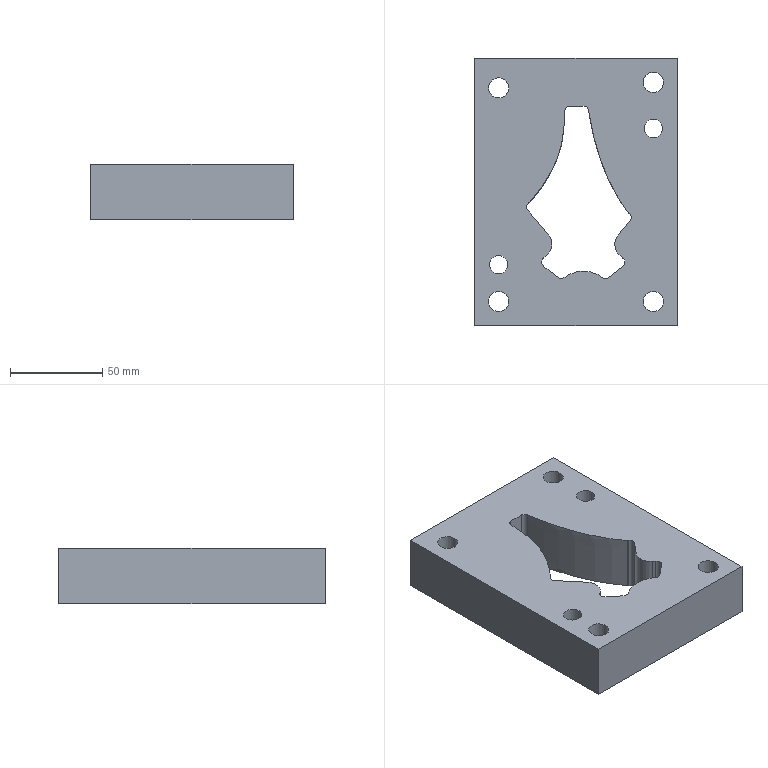Part | STEP file | 205_id718_x_t | 1 solid | 47 faces | box 110 x 145 x 30 mm | volume 364323 mm3 | cylinder 25 | plane 19 | other 3 | commonest cylinder face diameters 5 x8 11 x6 17 x4 6 x2 10 x2 16 x2